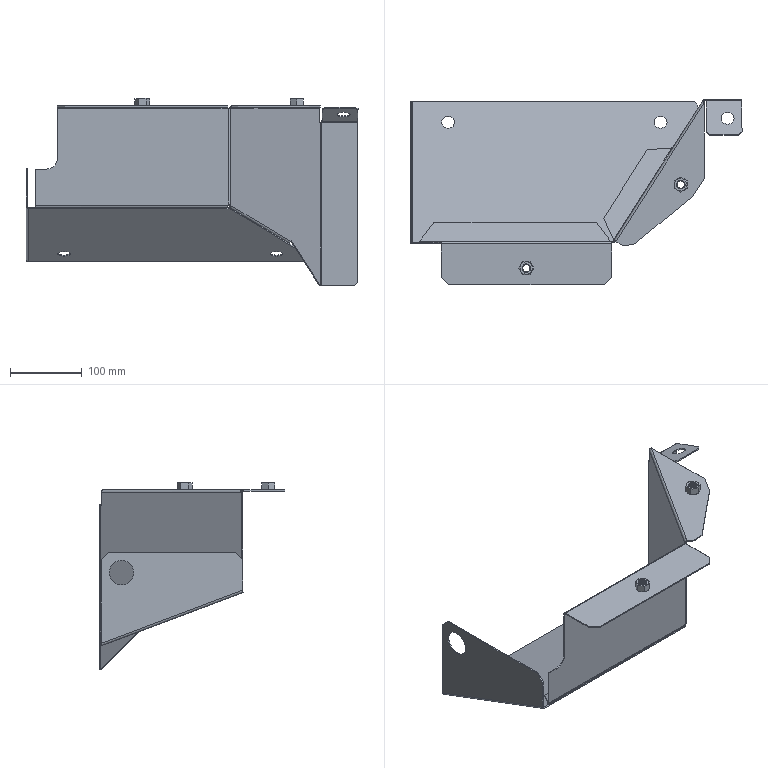Part | SolidWorks | 4 solids | 260 faces | box 461.2 x 257.358 x 260.639 mm | volume 345314 mm3 | plane 88 | cone 88 | cylinder 69 | spline 15 | commonest cylinder face diameters 10.106 x32 3 x8 6.2 x8 5 x7 18 x6 15 x4